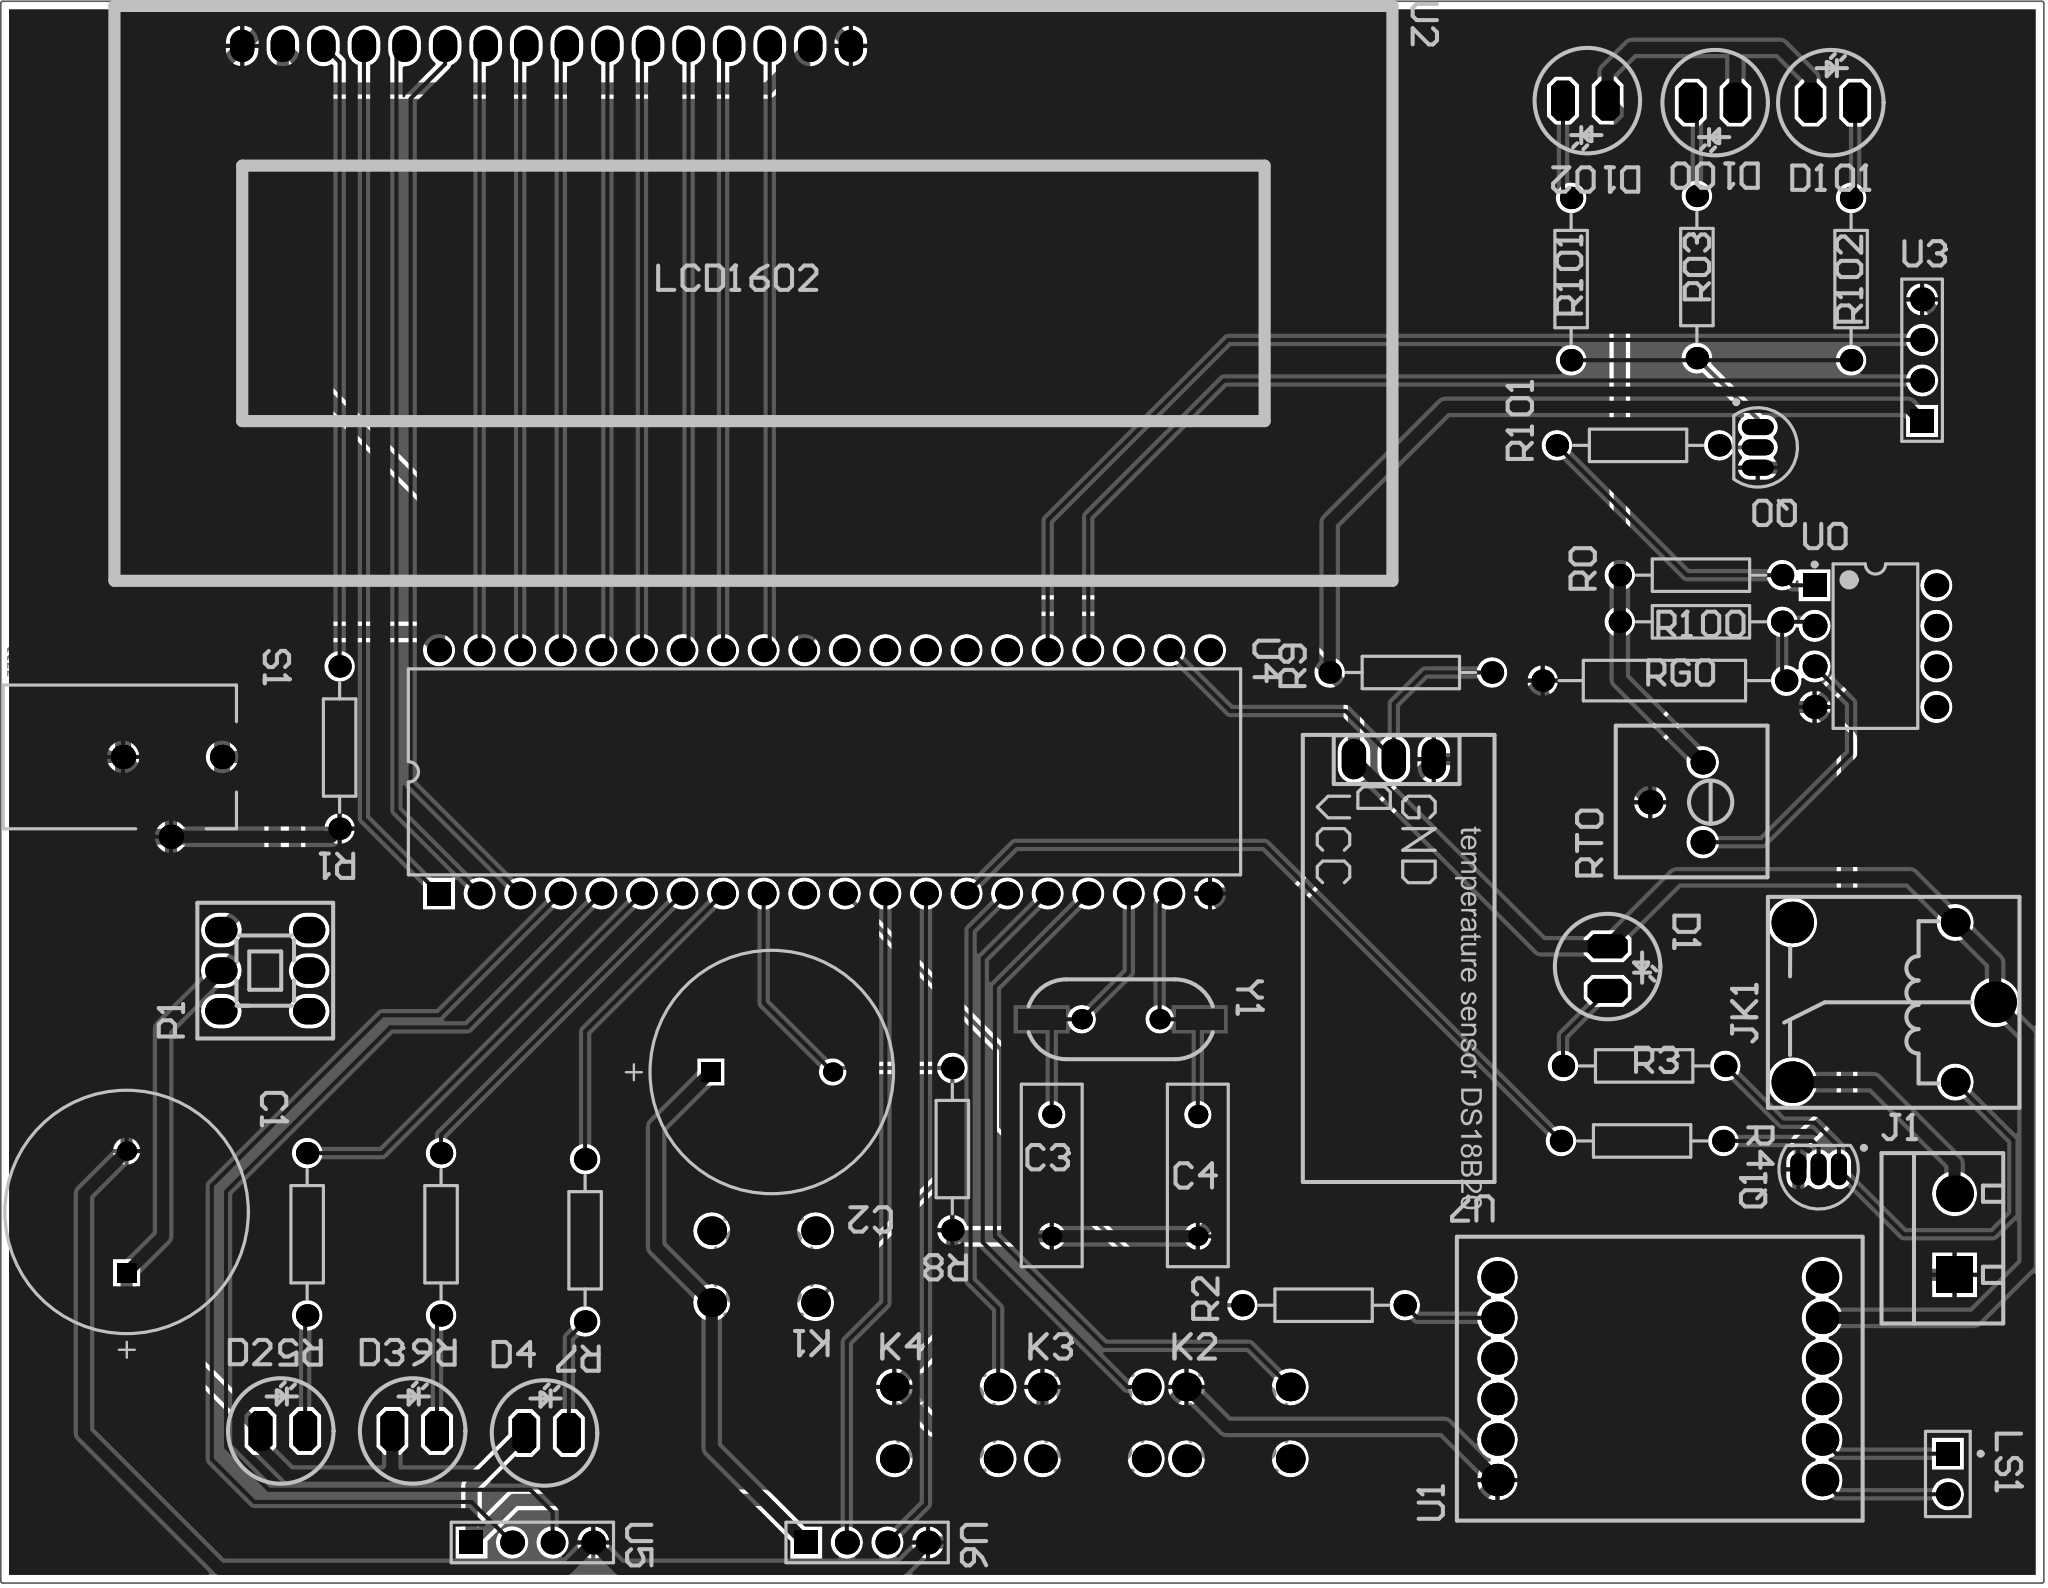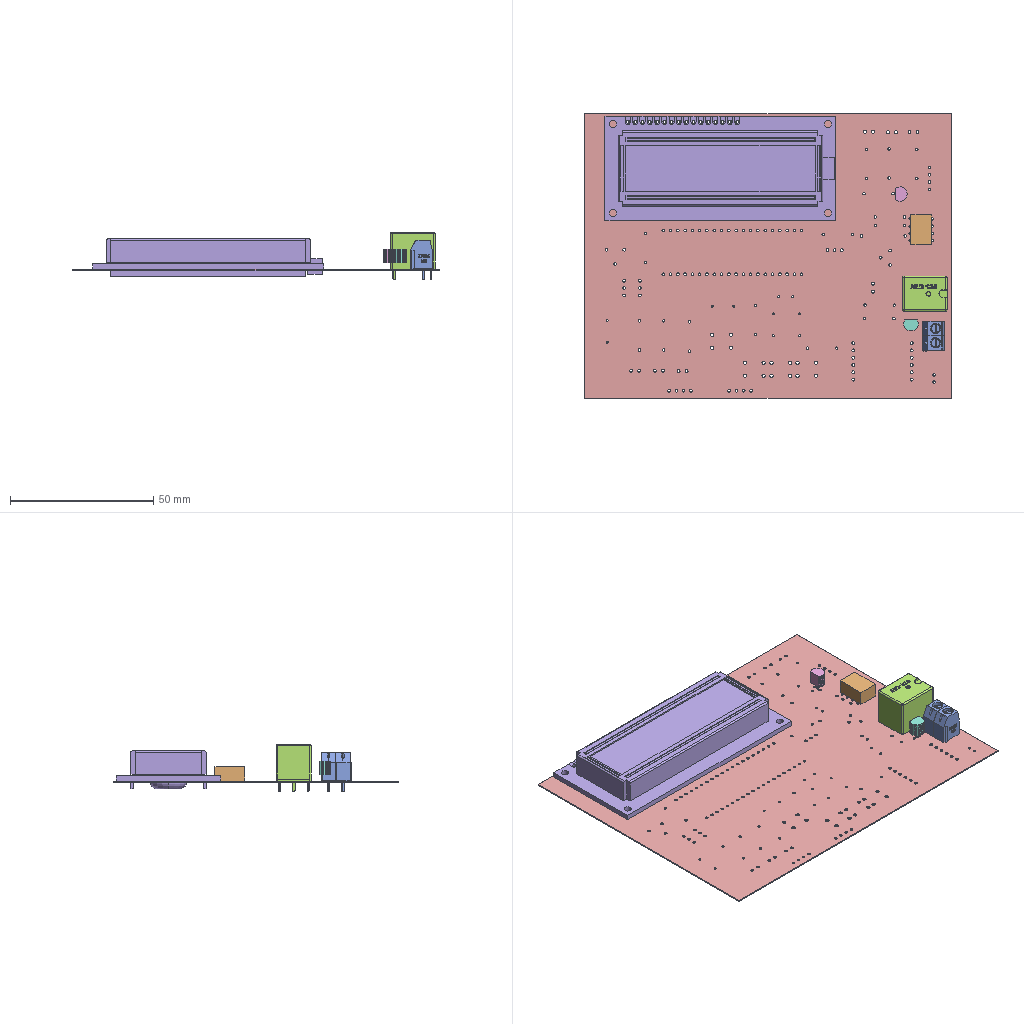Circuit board layout | Altium Designer | box 127.9 x 99.1 x 16.7 mm
Layer stack:
# Altium Designer layer stack of  (unit mm; dielectric type: 0 none, 1 core, 2 prepreg, 3 surface material)
index,name,kind,layer,copper_thickness_mm,dielectric_type,dielectric_thickness_mm,dielectric_material,dielectric_constant
0,Top Paste,other,,,,,,
1,Top Overlay,other,,,,,,
2,Top Solder,dielectric,,,3,0.0102,Solder Resist,3.5
3,Top Layer,copper,Top Layer,0.0356,,,,
4,Dielectric 1,dielectric,,,0,0.32,FR-4,4.8
5,Bottom Layer,copper,Bottom Layer,0.0356,,,,
6,Bottom Solder,dielectric,,,3,0.0102,Solder Resist,3.5
7,Bottom Overlay,other,,,,,,
8,Bottom Paste,other,,,,,,
# drill layer pairs: low layer,high layer
drill_pair,Top Layer,Bottom Layer
Part placement:
Designator,Comment,Layer,Footprint,Center-X(mm),Center-Y(mm),Rotation
C1,470uf,TopLayer,RB7.6-15,48.895,48.514,270
C2,10uf,TopLayer,RB7.6-15,89.281,57.277,180
C3,22PF,TopLayer,RAD-0.3,106.807,50.8,90
C4,22PF,TopLayer,RAD-0.3,115.951,50.8,90
D1,LED-R,TopLayer,LED,141.605,63.754,270
D2,LED-G,TopLayer,LED,58.674,34.798,0
D3,LED-R,TopLayer,LED,66.929,34.798,0
D4,LED-Y,TopLayer,LED,75.184,34.671,0
D100,white LED,TopLayer,LED,148.209,117.983,180
D101,white LED,TopLayer,LED,155.702,117.983,0
D102,white LED,TopLayer,LED,140.208,118.11,180
J1,,TopLayer,KF301-5.0-2P,163.322,47.117,90
JK1,HFKW-012-1ZW,TopLayer,012-1ZW_W,159.512,61.642,180
K1,push button,TopLayer,四脚轻触开关,88.773,45.085,180
K2,push button,TopLayer,四脚轻触开关,118.491,35.306,0
K3,push button,TopLayer,四脚轻触开关,109.474,35.306,0
K4,push button,TopLayer,四脚轻触开关,100.203,35.306,0
LS1,passive buzzer,TopLayer,PIN2,162.902,32.104,270
P1,latching switch,TopLayer,自锁开关,57.575,63.627,90
Q0,9012,TopLayer,TO-92A,151.003,96.393,180
Q1,9012,TopLayer,TO-92A,154.813,51.181,90
R0,10K,TopLayer,AXIAL-0.4,147.447,88.392,180
R1,2K,TopLayer,AXIAL-0.4,62.23,77.597,270
R2,1K,TopLayer,AXIAL-0.4,123.825,42.672,180
R03,1K,TopLayer,AXIAL-0.4,147.193,107.061,90
R3,1K,TopLayer,AXIAL-0.4,143.891,57.658,360
R4,1K,TopLayer,AXIAL-0.4,143.764,52.959,360
R5,1K,TopLayer,AXIAL-0.4,60.198,47.117,270
R6,1K,TopLayer,AXIAL-0.4,68.58,47.117,270
R7,1K,TopLayer,AXIAL-0.4,77.597,46.736,270
R8,10K,TopLayer,AXIAL-0.4,100.584,52.451,270
R9,10K,TopLayer,AXIAL-0.4,129.286,82.296,180
R100,10K,TopLayer,AXIAL-0.4,147.447,85.471,180
R101,1K,TopLayer,AXIAL-0.4,143.51,96.52,180
R101,1K,TopLayer,AXIAL-0.4,139.319,106.934,90
R102,1K,TopLayer,AXIAL-0.4,156.845,106.934,90
RG0,photoresistor,TopLayer,AXIAL-0.6,145.161,81.788,360
RT0,10K,TopLayer,电位器,145.913,74.168,90
S1,,TopLayer,KLD-0202,51.773,75.134,360
U0,LM393,TopLayer,DIP-8,158.369,83.947,0
U1,voice playback module-MY1680,TopLayer,MY1680,144.868,38.073,180
U2,LCD1602,TopLayer,LCD1602,75.184,121.539,360
U3,ultrasonic module,TopLayer,HDR1X4,161.29,101.854,90
U4,STC89C52,TopLayer,DIP-40,92.583,76.073,360
U5,ultrasonic module,TopLayer,HDR1X4,74.295,27.813,360
U6,ultrasonic module,TopLayer,HDR1X4,95.25,27.813,360
U7,DS18B20,TopLayer,DS18B20,128.222,76.869,270
Y1,11.059MHz,TopLayer,XTAL_US,111.122,60.579,360
Pad and via stacks:
# Altium Designer via and pad stacks of  (unit mm). Each distinct definition once, with the count of objects using it.
# via: kind,start_layer,end_layer,hole_mm,diameter_mm,mode(0 simple;1 top-mid-bottom;2 full stack),diameter_per_layer,count,example_net
# pad: kind,layer,hole_mm,hole_type(0 round;1 square;2 slot),plating,top_size,top_shape(1 round;2 rect;3 octagon;9 rounded rect),mid_size,bottom_size,mode,footprint,size_per_layer,count,example
pad,Multi-Layer,0.85,0,plated,1.4x1.4,1,1.4x1.4,1.4x1.4,0,AXIAL-0.6,,2,RG0.1
pad,Multi-Layer,0.9,0,plated,1.524x1.524,1,1.524x1.524,1.524x1.524,0,\u00B5\u00E7\u00CE\u00BB\u00C6\u00F7,,3,RT0.3
pad,Multi-Layer,0.9,0,plated,1.5x1.5,1,1.5x1.5,1.5x1.5,0,DIP-8,,7,U0.5
pad,Multi-Layer,0.9,0,plated,1.5x1.5,2,1.5x1.5,1.5x1.5,0,DIP-8,,1,U0.1
pad,Multi-Layer,0.9,0,plated,1.5x1.5,2,1.5x1.5,1.5x1.5,0,HDR1X4,,3,U6.1
pad,Multi-Layer,0.9,0,plated,1.5x1.5,1,1.5x1.5,1.5x1.5,0,HDR1X4,,9,U6.2
pad,Multi-Layer,0.85,0,plated,1.4x1.4,1,1.4x1.4,1.4x1.4,0,AXIAL-0.4,,30,R0.2
pad,Multi-Layer,0.7,0,plated,1.2x1.2,1,1.2x1.2,1.2x1.2,0,RAD-0.3,,4,C4.1
pad,Multi-Layer,0.7112,0,plated,1.27x1.27,1,1.27x1.27,1.27x1.27,0,XTAL_US,,2,Y1.1
pad,Multi-Layer,1.2,0,plated,1.8x1.8,1,1.8x1.8,1.8x1.8,0,\u00CB\u00C4\u00BD\u00C5\u00C7\u00E1\u00B4\u00A5\u00BF\u00AA\u00B9\u00D8,,16,K4.1
pad,Multi-Layer,0.9,0,plated,2x1,1,2x1,2x1,0,TO-92A,,6,Q0.1
pad,Multi-Layer,0.9,2,plated,2.524x1.524,1,2.524x1.524,2.524x1.524,0,DS18B20,,3,U7.1
pad,Multi-Layer,1,0,plated,1.5x2.5,3,1.5x2.5,1.5x2.5,0,LED,,14,D102.1
pad,Multi-Layer,0.7,0,plated,1.2x1.2,1,1.2x1.2,1.2x1.2,0,RB7.6-15,,2,C2.2
pad,Multi-Layer,0.7,0,plated,1.2x1.2,2,1.2x1.2,1.2x1.2,0,RB7.6-15,,2,C2.1
pad,Multi-Layer,0.9,0,plated,1.5x1.5,2,1.5x1.5,1.5x1.5,0,DIP-40,,1,U4.1
pad,Multi-Layer,0.9,0,plated,1.5x1.5,1,1.5x1.5,1.5x1.5,0,DIP-40,,39,U4.2
pad,Multi-Layer,1.2,0,plated,2.3x2.3,1,2.3x2.3,2.3x2.3,0,KF301-5.0-2P,,1,J1.2
pad,Multi-Layer,1.2,0,plated,2.3x2.3,2,2.3x2.3,2.3x2.3,0,KF301-5.0-2P,,1,J1.1
pad,Multi-Layer,0.9,0,plated,1.524x2.032,1,1.524x2.032,1.524x2.032,0,LCD1602,,16,U2.6
pad,Multi-Layer,0.9144,0,plated,1.651x2.032,1,1.651x2.032,1.651x2.032,0,\u00D7\u00D4\u00CB\u00F8\u00BF\u00AA\u00B9\u00D8,,6,P1.6
pad,Multi-Layer,1.6,0,plated,2.6x2.6,1,2.6x2.6,2.6x2.6,0,012-1ZW_W,,3,JK1.3
pad,Multi-Layer,1,0,plated,1.8x1.8,1,1.8x1.8,1.8x1.8,0,012-1ZW_W,,2,JK1.1
pad,Multi-Layer,0,0,plated,0x1.5,1,0x1.5,0x1.5,0,KLD-0202,,4,S1.1A
pad,Multi-Layer,0,0,plated,0x0,1,0x0,0x0,0,KLD-0202,,2,S1.2B
pad,Multi-Layer,1.016,0,plated,1.524x1.524,1,1.524x1.524,1.524x1.524,0,KLD-0202,,3,S1.3
pad,Multi-Layer,0.9,0,plated,1.5x1.5,1,1.5x1.5,1.5x1.5,0,PIN2,,1,LS1.2
pad,Multi-Layer,0.9,0,plated,1.5x1.5,2,1.5x1.5,1.5x1.5,0,PIN2,,1,LS1.1
pad,Multi-Layer,1.016,2,plated,2.032x2.032,1,2.032x2.032,2.032x2.032,0,MY1680,,12,U1.12
pad,Top Layer,0,0,plated,3x1.27,2,3x1.27,3x1.27,0,XTAL_US,,2,Y1.1
Copper pours:
name,layer,net,type(0 solid;1 hatched;2 none)
Top Layer-No Net,Top Layer,GND,0
Top Layer-No Net,Bottom Layer,GND,0
Design rules, without the lines most boards share:
# Altium Designer design rules of  (exported by Altium Designer, unit mm)
# columns: name | kind | enabled | priority | scope1 | scope2 | descriptor | typed fields (field=value)
Clearance | 0 | enabled | 1 | All | All | Clearance Constraint (Gap=10mil) (All),(All) | gap=0.254
PlaneConnect | 6 | enabled | 1 | All | All | Power Plane Connect Rule(Relief Connect )(Expansion=20mil) (Conductor Width=10mil) (Air Gap=10mil) (Entries=4) (All) | relief_conductor_width=0.254 relief_entries=4 relief_expansion=0.508
PolygonConnect | 20 | enabled | 1 | All | All | Polygon Connect Rule(Relief Connect )(Conductor Width=10mil) (Relief Angle=90 Angle) (Entries=4) (Air Gap Width=10mil) (All),(All) | connect_style(0=relief,1=direct,2=none)=0 relief_conductor_width=0.254 relief_entries=4
Width | 2 | enabled | 1 | All | All | Width Constraint (Min=10mil) (Max=30mil) (Preferred=10mil) (All) |
RoutingVias | 11 | enabled | 1 | All | All | Routing Via (MinHoleWidth=28mil) (MaxHoleWidth=28mil) (PreferredHoleWidth=28mil) (MinWidth=50mil) (MaxWidth=50mil) (PreferedWidth=50mil) (All) | via_min_hole=0.7112 via_max_hole=0.7112 via_preferred_diameter=1.27 via_preferred_hole=0.7112
PasteMaskExpansion | 14 | enabled | 1 | All | All | Paste Mask Expansion (Expansion =0mil) (All) | expansion=0
SolderMaskExpansion | 13 | enabled | 1 | All | All | Solder Mask Expansion (Expansion =4mil) (All) | expansion=0.1016
DiffPairsRouting | 51 | enabled | 1 | All | All | Differential Pairs Uncoupled Length using the Gap Constraints (Min=10mil) (Max=10mil) (Prefered=10mil)  and Width Constraints (Min=15mil) (Max=15mil) (Prefered=15mil) (All) |
HoleToHoleClearance | 52 | enabled | 1 | All | All | Hole To Hole Clearance (Gap=10mil) (All),(All) | gap=0.254
MinimumSolderMaskSliver | 53 | enabled | 1 | All | All | Minimum Solder Mask Sliver (Gap=0mil) (All),(All) |
SilkToSolderMaskClearance | 54 | enabled | 1 | IsPad | All | Silk To Solder Mask (Clearance=0mil) (IsPad),(All) |
SilkToSilkClearance | 55 | enabled | 1 | All | All | Silk to Silk (Clearance=0mil) (All),(All) |